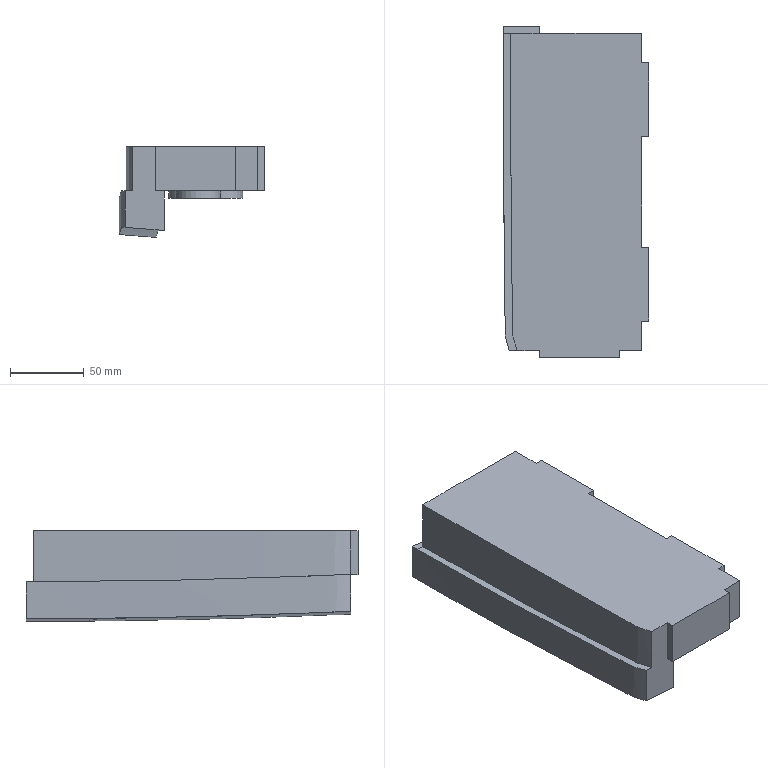Part | NX | features solid 2 | 1 solid | 37 faces | box 98.803 x 225 x 61.502 mm | volume 766581 mm3 | plane 22 | spline 10 | cylinder 5 | commonest cylinder face diameters 30 x5